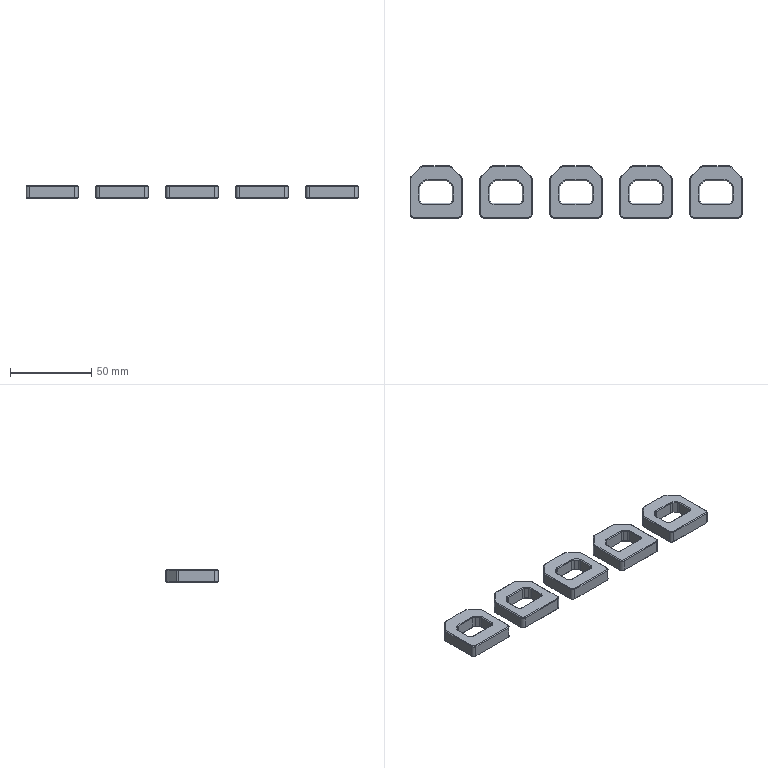NC program | NX | posted with a generic post | part box 204 x 32 x 8 mm
Lines 19 to 988 of 9506:
(ZLEVEL_PROFILE_COPY_1 , TOOL : D10)
N36 T15 M6
N38 G54
N40 G17 G0 G90 X4.9 Y-0.132 S9500 M3
N42 G43 Z30. H15
N44 Z1.5
N46 G94 G1 Y1.888 Z1.394 F1000.
N48 X4.888 Y1.9 Z1.393
N50 X-4.888 Z0.881
N52 X-4.9 Y1.888 Z0.88
N54 Y-1.9 Z0.682
N56 X4.9 Z0.168
N58 Y1.888 Z-0.031
N60 X4.888 Y1.9
N62 X-4.888 Z-0.544
N64 X-4.9 Y1.888 Z-0.545
N66 Y-1.9 Z-0.743
N68 X0. Z-1.
N70 X4.9 F3500.
N72 Y1.888
N74 X4.888 Y1.9
N76 X-4.888
N78 X-4.9 Y1.888
N80 Y-1.9
N82 X0.
N84 X4.9 Z-1.18
N86 Y0.001 Z-1.25
N88 X4.888 Y1.9 Z-1.32
N90 X-4.888 Z-1.68
N92 X-4.9 Y0.635 Z-1.56
N94 Y0. Z-1.5
N96 Y-1.9 Z-1.82
N98 X0. Z-2.
N100 X4.9 Z-2.18
N102 Y0.001 Z-2.25
N104 X4.888 Y1.9 Z-2.32
N106 X-4.888 Z-2.68
N108 X-4.9 Y0.635 Z-2.56
N110 Y0. Z-2.5
N112 Y-1.9 Z-2.82
N114 X0. Z-3.
N116 X4.9 Z-3.18
N118 Y0.001 Z-3.25
N120 X4.888 Y1.9 Z-3.32
N122 X-4.888 Z-3.68
N124 X-4.9 Y0.635 Z-3.56
N126 Y0. Z-3.5
N128 Y-1.9 Z-3.82
N130 X0. Z-4.
N132 X4.9 Z-4.18
N134 Y0.001 Z-4.25
N136 X4.888 Y1.9 Z-4.32
N138 X-4.888 Z-4.68
N140 X-4.9 Y0.635 Z-4.56
N142 Y0. Z-4.5
N144 Y-1.9 Z-4.82
N146 X0. Z-5.
N148 X4.9 Z-5.18
N150 Y0.001 Z-5.25
N152 X4.888 Y1.9 Z-5.32
N154 X-4.888 Z-5.68
N156 X-4.9 Y0.635 Z-5.56
N158 Y0. Z-5.5
N160 Y-1.9 Z-5.82
N162 X0. Z-6.
N164 X4.9 Z-6.18
N166 Y0.001 Z-6.25
N168 X4.888 Y1.9 Z-6.32
N170 X-4.888 Z-6.68
N172 X-4.9 Y0.635 Z-6.56
N174 Y0. Z-6.5
N176 Y-1.9 Z-6.82
N178 X0. Z-7.
N180 X4.9 Z-7.18
N182 Y0.001 Z-7.25
N184 X4.888 Y1.9 Z-7.32
N186 X-4.888 Z-7.68
N188 X-4.9 Y0.635 Z-7.56
N190 Y0. Z-7.5
N192 Y-1.9 Z-7.82
N194 X0. Z-8.
N196 X4.9
N198 Y1.888
N200 X4.888 Y1.9
N202 X-4.888
N204 X-4.9 Y1.888
N206 Y-1.9
N208 X0.
N210 Z-6.5
N212 G0 Z53.
N214 X-38.1 Y-0.132
N216 Z1.5
N218 G1 Y1.888 Z1.394 F1000.
N220 X-38.112 Y1.9 Z1.393
N222 X-47.888 Z0.881
N224 X-47.9 Y1.888 Z0.88
N226 Y-1.9 Z0.682
N228 X-38.1 Z0.168
N230 Y1.888 Z-0.031
N232 X-38.112 Y1.9
N234 X-47.888 Z-0.544
N236 X-47.9 Y1.888 Z-0.545
N238 Y-1.9 Z-0.743
N240 X-43. Z-1.
N242 X-38.1 F3500.
N244 Y1.888
N246 X-38.112 Y1.9
N248 X-47.888
N250 X-47.9 Y1.888
N252 Y-1.9
N254 X-43.
N256 X-38.1 Z-1.18
N258 Y0.002 Z-1.25
N260 X-38.112 Y1.901 Z-1.32
N262 X-47.888 Y1.9 Z-1.68
N264 X-47.9 Y0.635 Z-1.726
N266 Y-1.9 Z-1.82
N268 X-43. Z-2.
N270 X-38.1 Z-2.18
N272 Y0.002 Z-2.25
N274 X-38.112 Y1.901 Z-2.32
N276 X-47.888 Y1.9 Z-2.68
N278 X-47.9 Y0.635 Z-2.726
N280 Y-1.9 Z-2.82
N282 X-43. Z-3.
N284 X-38.1 Z-3.18
N286 Y0.002 Z-3.25
N288 X-38.112 Y1.901 Z-3.32
N290 X-47.888 Y1.9 Z-3.68
N292 X-47.9 Y0.635 Z-3.726
N294 Y-1.9 Z-3.82
N296 X-43. Z-4.
N298 X-38.1 Z-4.18
N300 Y0.002 Z-4.25
N302 X-38.112 Y1.901 Z-4.32
N304 X-47.888 Y1.9 Z-4.68
N306 X-47.9 Y0.635 Z-4.726
N308 Y-1.9 Z-4.82
N310 X-43. Z-5.
N312 X-38.1 Z-5.18
N314 Y0.002 Z-5.25
N316 X-38.112 Y1.901 Z-5.32
N318 X-47.888 Y1.9 Z-5.68
N320 X-47.9 Y0.635 Z-5.726
N322 Y-1.9 Z-5.82
N324 X-43. Z-6.
N326 X-38.1 Z-6.18
N328 Y0.002 Z-6.25
N330 X-38.112 Y1.901 Z-6.32
N332 X-47.888 Y1.9 Z-6.68
N334 X-47.9 Y0.635 Z-6.726
N336 Y-1.9 Z-6.82
N338 X-43. Z-7.
N340 X-38.1 Z-7.18
N342 Y0.002 Z-7.25
N344 X-38.112 Y1.901 Z-7.32
N346 X-47.888 Y1.9 Z-7.68
N348 X-47.9 Y0.635 Z-7.726
N350 Y-1.9 Z-7.82
N352 X-43. Z-8.
N354 X-38.1
N356 Y1.888
N358 X-38.112 Y1.9
N360 X-47.888
N362 X-47.9 Y1.888
N364 Y-1.9
N366 X-43.
N368 Z-6.5
N370 G0 Z53.
N372 X-81.1 Y-0.132
N374 Z1.5
N376 G1 Y1.888 Z1.394 F1000.
N378 X-81.112 Y1.9 Z1.393
N380 X-90.888 Z0.881
N382 X-90.9 Y1.888 Z0.88
N384 Y-1.9 Z0.682
N386 X-81.1 Z0.168
N388 Y1.888 Z-0.031
N390 X-81.112 Y1.9
N392 X-90.888 Z-0.544
N394 X-90.9 Y1.888 Z-0.545
N396 Y-1.9 Z-0.743
N398 X-86. Z-1.
N400 X-81.1 F3500.
N402 Y1.888
N404 X-81.112 Y1.9
N406 X-90.888
N408 X-90.9 Y1.888
N410 Y-1.9
N412 X-86.
N414 X-81.1 Z-1.18
N416 Y0.001 Z-1.25
N418 X-81.112 Y1.9 Z-1.32
N420 X-90.888 Z-1.68
N422 X-90.9 Y0.635 Z-1.56
N424 Y0. Z-1.5
N426 Y-1.9 Z-1.82
N428 X-86. Z-2.
N430 X-81.1 Z-2.18
N432 Y0.001 Z-2.25
N434 X-81.112 Y1.9 Z-2.32
N436 X-90.888 Z-2.68
N438 X-90.9 Y0.635 Z-2.56
N440 Y0. Z-2.5
N442 Y-1.9 Z-2.82
N444 X-86. Z-3.
N446 X-81.1 Z-3.18
N448 Y0.001 Z-3.25
N450 X-81.112 Y1.9 Z-3.32
N452 X-90.888 Z-3.68
N454 X-90.9 Y0.635 Z-3.56
N456 Y0. Z-3.5
N458 Y-1.9 Z-3.82
N460 X-86. Z-4.
N462 X-81.1 Z-4.18
N464 Y0.001 Z-4.25
N466 X-81.112 Y1.9 Z-4.32
N468 X-90.888 Z-4.68
N470 X-90.9 Y0.635 Z-4.56
N472 Y0. Z-4.5
N474 Y-1.9 Z-4.82
N476 X-86. Z-5.
N478 X-81.1 Z-5.18
N480 Y0.001 Z-5.25
N482 X-81.112 Y1.9 Z-5.32
N484 X-90.888 Z-5.68
N486 X-90.9 Y0.635 Z-5.56
N488 Y0. Z-5.5
N490 Y-1.9 Z-5.82
N492 X-86. Z-6.
N494 X-81.1 Z-6.18
N496 Y0.001 Z-6.25
N498 X-81.112 Y1.9 Z-6.32
N500 X-90.888 Z-6.68
N502 X-90.9 Y0.635 Z-6.56
N504 Y0. Z-6.5
N506 Y-1.9 Z-6.82
N508 X-86. Z-7.
N510 X-81.1 Z-7.18
N512 Y0.001 Z-7.25
N514 X-81.112 Y1.9 Z-7.32
N516 X-90.888 Z-7.68
N518 X-90.9 Y0.635 Z-7.56
N520 Y0. Z-7.5
N522 Y-1.9 Z-7.82
N524 X-86. Z-8.
N526 X-81.1
N528 Y1.888
N530 X-81.112 Y1.9
N532 X-90.888
N534 X-90.9 Y1.888
N536 Y-1.9
N538 X-86.
N540 Z-6.5
N542 G0 Z53.
N544 X90.9 Y-0.132
N546 Z1.5
N548 G1 Y1.888 Z1.394 F1000.
N550 X90.888 Y1.9 Z1.393
N552 X81.112 Z0.881
N554 X81.1 Y1.888 Z0.88
N556 Y-1.9 Z0.682
N558 X90.9 Z0.168
N560 Y1.888 Z-0.031
N562 X90.888 Y1.9
N564 X81.112 Z-0.544
N566 X81.1 Y1.888 Z-0.545
N568 Y-1.9 Z-0.743
N570 X86. Z-1.
N572 X90.9 F3500.
N574 Y1.888
N576 X90.888 Y1.9
N578 X81.112
N580 X81.1 Y1.888
N582 Y-1.9
N584 X86.
N586 X90.9 Z-1.18
N588 Y0.002 Z-1.25
N590 X90.888 Y1.901 Z-1.32
N592 X81.112 Y1.9 Z-1.68
N594 X81.1 Y0.635 Z-1.726
N596 Y-1.9 Z-1.82
N598 X86. Z-2.
N600 X90.9 Z-2.18
N602 Y0.002 Z-2.25
N604 X90.888 Y1.901 Z-2.32
N606 X81.112 Y1.9 Z-2.68
N608 X81.1 Y0.635 Z-2.726
N610 Y-1.9 Z-2.82
N612 X86. Z-3.
N614 X90.9 Z-3.18
N616 Y0.002 Z-3.25
N618 X90.888 Y1.901 Z-3.32
N620 X81.112 Y1.9 Z-3.68
N622 X81.1 Y0.635 Z-3.726
N624 Y-1.9 Z-3.82
N626 X86. Z-4.
N628 X90.9 Z-4.18
N630 Y0.002 Z-4.25
N632 X90.888 Y1.901 Z-4.32
N634 X81.112 Y1.9 Z-4.68
N636 X81.1 Y0.635 Z-4.726
N638 Y-1.9 Z-4.82
N640 X86. Z-5.
N642 X90.9 Z-5.18
N644 Y0.002 Z-5.25
N646 X90.888 Y1.901 Z-5.32
N648 X81.112 Y1.9 Z-5.68
N650 X81.1 Y0.635 Z-5.726
N652 Y-1.9 Z-5.82
N654 X86. Z-6.
N656 X90.9 Z-6.18
N658 Y0.002 Z-6.25
N660 X90.888 Y1.901 Z-6.32
N662 X81.112 Y1.9 Z-6.68
N664 X81.1 Y0.635 Z-6.726
N666 Y-1.9 Z-6.82
N668 X86. Z-7.
N670 X90.9 Z-7.18
N672 Y0.002 Z-7.25
N674 X90.888 Y1.901 Z-7.32
N676 X81.112 Y1.9 Z-7.68
N678 X81.1 Y0.635 Z-7.726
N680 Y-1.9 Z-7.82
N682 X86. Z-8.
N684 X90.9
N686 Y1.888
N688 X90.888 Y1.9
N690 X81.112
N692 X81.1 Y1.888
N694 Y-1.9
N696 X86.
N698 Z-6.5
N700 G0 Z53.
N702 X47.9 Y-0.132
N704 Z1.5
N706 G1 Y1.888 Z1.394 F1000.
N708 X47.888 Y1.9 Z1.393
N710 X38.112 Z0.881
N712 X38.1 Y1.888 Z0.88
N714 Y-1.9 Z0.682
N716 X47.9 Z0.168
N718 Y1.888 Z-0.031
N720 X47.888 Y1.9
N722 X38.112 Z-0.544
N724 X38.1 Y1.888 Z-0.545
N726 Y-1.9 Z-0.743
N728 X43. Z-1.
N730 X47.9 F3500.
N732 Y1.888
N734 X47.888 Y1.9
N736 X38.112
N738 X38.1 Y1.888
N740 Y-1.9
N742 X43.
N744 X47.9 Z-1.18
N746 Y0.002 Z-1.25
N748 X47.888 Y1.901 Z-1.32
N750 X38.112 Y1.9 Z-1.68
N752 X38.1 Y0.635 Z-1.726
N754 Y-1.9 Z-1.82
N756 X43. Z-2.
N758 X47.9 Z-2.18
N760 Y0.002 Z-2.25
N762 X47.888 Y1.901 Z-2.32
N764 X38.112 Y1.9 Z-2.68
N766 X38.1 Y0.635 Z-2.726
N768 Y-1.9 Z-2.82
N770 X43. Z-3.
N772 X47.9 Z-3.18
N774 Y0.002 Z-3.25
N776 X47.888 Y1.901 Z-3.32
N778 X38.112 Y1.9 Z-3.68
N780 X38.1 Y0.635 Z-3.726
N782 Y-1.9 Z-3.82
N784 X43. Z-4.
N786 X47.9 Z-4.18
N788 Y0.002 Z-4.25
N790 X47.888 Y1.901 Z-4.32
N792 X38.112 Y1.9 Z-4.68
N794 X38.1 Y0.635 Z-4.726
N796 Y-1.9 Z-4.82
N798 X43. Z-5.
N800 X47.9 Z-5.18
N802 Y0.002 Z-5.25
N804 X47.888 Y1.901 Z-5.32
N806 X38.112 Y1.9 Z-5.68
N808 X38.1 Y0.635 Z-5.726
N810 Y-1.9 Z-5.82
N812 X43. Z-6.
N814 X47.9 Z-6.18
N816 Y0.002 Z-6.25
N818 X47.888 Y1.901 Z-6.32
N820 X38.112 Y1.9 Z-6.68
N822 X38.1 Y0.635 Z-6.726
N824 Y-1.9 Z-6.82
N826 X43. Z-7.
N828 X47.9 Z-7.18
N830 Y0.002 Z-7.25
N832 X47.888 Y1.901 Z-7.32
N834 X38.112 Y1.9 Z-7.68
N836 X38.1 Y0.635 Z-7.726
N838 Y-1.9 Z-7.82
N840 X43. Z-8.
N842 X47.9
N844 Y1.888
N846 X47.888 Y1.9
N848 X38.112
N850 X38.1 Y1.888
N852 Y-1.9
N854 X43.
N856 Z-6.5
N858 G0 Z53.
N860 X64.1 Y8.527
N862 Z1.5
N864 G1 Y-14.653 Z0.285 F1000.
N866 X63.761 Y-16.263 Z0.199
N868 X63.063 Y-17.752 Z0.113
N870 X62.042 Y-19.042 Z0.027
N872 X60.752 Y-20.063 Z-0.06
N874 X59.263 Y-20.761 Z-0.146
N876 X57.653 Y-21.1 Z-0.232
N878 X43. Z-1.
N880 X29. F3500.
N882 G2 X21.9 Y-14. R7.1
N884 G1 Y8.172
N886 G2 X23.98 Y13.192 R7.1
N888 G1 X29.808 Y19.02
N890 G2 X34.828 Y21.1 R7.1
N892 G1 X51.172
N894 G2 X56.192 Y19.02 R7.1
N896 G1 X62.02 Y13.192
N898 G2 X64.1 Y8.172 R7.1
N900 G1 Y-14.
N902 G2 X57. Y-21.1 R7.1
N904 G1 X43.
N906 X29. Z-1.094
N908 X28.381 Y-21.073 Z-1.098
N910 X27.767 Y-20.992 Z-1.102
N912 X27.162 Y-20.858 Z-1.106
N914 X26.572 Y-20.672 Z-1.11
N916 X25.999 Y-20.435 Z-1.114
N918 X25.45 Y-20.149 Z-1.118
N920 X24.928 Y-19.816 Z-1.122
N922 X24.436 Y-19.439 Z-1.127
N924 X23.98 Y-19.02 Z-1.131
N926 X23.561 Y-18.564 Z-1.135
N928 X23.184 Y-18.072 Z-1.139
N930 X22.851 Y-17.55 Z-1.143
N932 X22.565 Y-17.001 Z-1.147
N934 X22.328 Y-16.428 Z-1.151
N936 X22.142 Y-15.838 Z-1.155
N938 X22.008 Y-15.233 Z-1.16
N940 X21.927 Y-14.619 Z-1.164
N942 X21.9 Y-14. Z-1.168
N944 Y8.172 Z-1.316
N946 X21.922 Y8.729 Z-1.32
N948 X21.987 Y9.282 Z-1.323
N950 X22.096 Y9.829 Z-1.327
N952 X22.247 Y10.366 Z-1.331
N954 X22.44 Y10.889 Z-1.335
N956 X22.674 Y11.395 Z-1.338
N958 X22.946 Y11.881 Z-1.342
N960 X23.256 Y12.345 Z-1.346
N962 X23.601 Y12.783 Z-1.349
N964 X23.98 Y13.192 Z-1.353
N966 X29.808 Y19.02 Z-1.408
N968 X30.217 Y19.399 Z-1.412
N970 X30.655 Y19.744 Z-1.416
N972 X31.119 Y20.054 Z-1.419
N974 X31.605 Y20.326 Z-1.423
N976 X32.111 Y20.56 Z-1.427
N978 X32.634 Y20.753 Z-1.431
N980 X33.171 Y20.904 Z-1.434
N982 X33.718 Y21.013 Z-1.438
N984 X34.271 Y21.078 Z-1.442
N986 X34.828 Y21.1 Z-1.445
N988 X51.172 Z-1.555
N990 X51.729 Y21.078 Z-1.558
N992 X52.282 Y21.013 Z-1.562
N994 X52.829 Y20.904 Z-1.566
N996 X53.366 Y20.753 Z-1.569
N998 X53.889 Y20.56 Z-1.573
N1000 X54.395 Y20.326 Z-1.577
N1002 X54.881 Y20.054 Z-1.581
N1004 X55.345 Y19.744 Z-1.584
N1006 X55.783 Y19.399 Z-1.588
N1008 X56.192 Y19.02 Z-1.592
N1010 X62.02 Y13.192 Z-1.647
N1012 X62.399 Y12.783 Z-1.651
N1014 X62.744 Y12.345 Z-1.654
N1016 X63.054 Y11.881 Z-1.658
N1018 X63.326 Y11.395 Z-1.662
N1020 X63.56 Y10.889 Z-1.665
N1022 X63.753 Y10.366 Z-1.669
N1024 X63.904 Y9.829 Z-1.673
N1026 X64.013 Y9.282 Z-1.677
N1028 X64.078 Y8.729 Z-1.68
N1030 X64.1 Y8.172 Z-1.684
N1032 Y-14. Z-1.832
N1034 X64.073 Y-14.619 Z-1.836
N1036 X63.992 Y-15.233 Z-1.84
N1038 X63.858 Y-15.838 Z-1.845
N1040 X63.672 Y-16.428 Z-1.849
N1042 X63.435 Y-17.001 Z-1.853
N1044 X63.149 Y-17.55 Z-1.857
N1046 X62.816 Y-18.072 Z-1.861
N1048 X62.439 Y-18.564 Z-1.865
N1050 X62.02 Y-19.02 Z-1.869
N1052 X61.564 Y-19.439 Z-1.873
N1054 X61.072 Y-19.816 Z-1.878
N1056 X60.55 Y-20.149 Z-1.882
N1058 X60.001 Y-20.435 Z-1.886
N1060 X59.428 Y-20.672 Z-1.89
N1062 X58.838 Y-20.858 Z-1.894
N1064 X58.233 Y-20.992 Z-1.898
N1066 X57.619 Y-21.073 Z-1.902
N1068 X57. Y-21.1 Z-1.906
N1070 X43. Z-2.
N1072 X29. Z-2.094
N1074 X28.381 Y-21.073 Z-2.098
N1076 X27.767 Y-20.992 Z-2.102
N1078 X27.162 Y-20.858 Z-2.106
N1080 X26.572 Y-20.672 Z-2.11
N1082 X25.999 Y-20.435 Z-2.114
N1084 X25.45 Y-20.149 Z-2.118
N1086 X24.928 Y-19.816 Z-2.122
N1088 X24.436 Y-19.439 Z-2.127
N1090 X23.98 Y-19.02 Z-2.131
N1092 X23.561 Y-18.564 Z-2.135
N1094 X23.184 Y-18.072 Z-2.139
N1096 X22.851 Y-17.55 Z-2.143
N1098 X22.565 Y-17.001 Z-2.147
N1100 X22.328 Y-16.428 Z-2.151
N1102 X22.142 Y-15.838 Z-2.155
N1104 X22.008 Y-15.233 Z-2.16
N1106 X21.927 Y-14.619 Z-2.164
N1108 X21.9 Y-14. Z-2.168
N1110 Y8.172 Z-2.316
N1112 X21.922 Y8.729 Z-2.32
N1114 X21.987 Y9.282 Z-2.323
N1116 X22.096 Y9.829 Z-2.327
N1118 X22.247 Y10.366 Z-2.331
N1120 X22.44 Y10.889 Z-2.335
N1122 X22.674 Y11.395 Z-2.338
N1124 X22.946 Y11.881 Z-2.342
N1126 X23.256 Y12.345 Z-2.346
N1128 X23.601 Y12.783 Z-2.349
N1130 X23.98 Y13.192 Z-2.353
N1132 X29.808 Y19.02 Z-2.408
N1134 X30.217 Y19.399 Z-2.412
N1136 X30.655 Y19.744 Z-2.416
N1138 X31.119 Y20.054 Z-2.419
N1140 X31.605 Y20.326 Z-2.423
N1142 X32.111 Y20.56 Z-2.427
N1144 X32.634 Y20.753 Z-2.431
N1146 X33.171 Y20.904 Z-2.434
N1148 X33.718 Y21.013 Z-2.438
N1150 X34.271 Y21.078 Z-2.442
N1152 X34.828 Y21.1 Z-2.445
N1154 X51.172 Z-2.555
N1156 X51.729 Y21.078 Z-2.558
N1158 X52.282 Y21.013 Z-2.562
N1160 X52.829 Y20.904 Z-2.566
N1162 X53.366 Y20.753 Z-2.569
N1164 X53.889 Y20.56 Z-2.573
N1166 X54.395 Y20.326 Z-2.577
N1168 X54.881 Y20.054 Z-2.581
N1170 X55.345 Y19.744 Z-2.584
N1172 X55.783 Y19.399 Z-2.588
N1174 X56.192 Y19.02 Z-2.592
N1176 X62.02 Y13.192 Z-2.647
N1178 X62.399 Y12.783 Z-2.651
N1180 X62.744 Y12.345 Z-2.654
N1182 X63.054 Y11.881 Z-2.658
N1184 X63.326 Y11.395 Z-2.662
N1186 X63.56 Y10.889 Z-2.665
N1188 X63.753 Y10.366 Z-2.669
N1190 X63.904 Y9.829 Z-2.673
N1192 X64.013 Y9.282 Z-2.677
N1194 X64.078 Y8.729 Z-2.68
N1196 X64.1 Y8.172 Z-2.684
N1198 Y-14. Z-2.832
N1200 X64.073 Y-14.619 Z-2.836
N1202 X63.992 Y-15.233 Z-2.84
N1204 X63.858 Y-15.838 Z-2.845
N1206 X63.672 Y-16.428 Z-2.849
N1208 X63.435 Y-17.001 Z-2.853
N1210 X63.149 Y-17.55 Z-2.857
N1212 X62.816 Y-18.072 Z-2.861
N1214 X62.439 Y-18.564 Z-2.865
N1216 X62.02 Y-19.02 Z-2.869
N1218 X61.564 Y-19.439 Z-2.873
N1220 X61.072 Y-19.816 Z-2.878
N1222 X60.55 Y-20.149 Z-2.882
N1224 X60.001 Y-20.435 Z-2.886
N1226 X59.428 Y-20.672 Z-2.89
N1228 X58.838 Y-20.858 Z-2.894
N1230 X58.233 Y-20.992 Z-2.898
N1232 X57.619 Y-21.073 Z-2.902
N1234 X57. Y-21.1 Z-2.906
N1236 X43. Z-3.
N1238 X29. Z-3.094
N1240 X28.381 Y-21.073 Z-3.098
N1242 X27.767 Y-20.992 Z-3.102
N1244 X27.162 Y-20.858 Z-3.106
N1246 X26.572 Y-20.672 Z-3.11
N1248 X25.999 Y-20.435 Z-3.114
N1250 X25.45 Y-20.149 Z-3.118
N1252 X24.928 Y-19.816 Z-3.122
N1254 X24.436 Y-19.439 Z-3.127
N1256 X23.98 Y-19.02 Z-3.131
N1258 X23.561 Y-18.564 Z-3.135
N1260 X23.184 Y-18.072 Z-3.139
N1262 X22.851 Y-17.55 Z-3.143
N1264 X22.565 Y-17.001 Z-3.147
N1266 X22.328 Y-16.428 Z-3.151
N1268 X22.142 Y-15.838 Z-3.155
N1270 X22.008 Y-15.233 Z-3.16
N1272 X21.927 Y-14.619 Z-3.164
N1274 X21.9 Y-14. Z-3.168
N1276 Y8.172 Z-3.316
N1278 X21.922 Y8.729 Z-3.32
N1280 X21.987 Y9.282 Z-3.323
N1282 X22.096 Y9.829 Z-3.327
N1284 X22.247 Y10.366 Z-3.331
N1286 X22.44 Y10.889 Z-3.335
N1288 X22.674 Y11.395 Z-3.338
N1290 X22.946 Y11.881 Z-3.342
N1292 X23.256 Y12.345 Z-3.346
N1294 X23.601 Y12.783 Z-3.349
N1296 X23.98 Y13.192 Z-3.353
N1298 X29.808 Y19.02 Z-3.408
N1300 X30.217 Y19.399 Z-3.412
N1302 X30.655 Y19.744 Z-3.416
N1304 X31.119 Y20.054 Z-3.419
N1306 X31.605 Y20.326 Z-3.423
N1308 X32.111 Y20.56 Z-3.427
N1310 X32.634 Y20.753 Z-3.431
N1312 X33.171 Y20.904 Z-3.434
N1314 X33.718 Y21.013 Z-3.438
N1316 X34.271 Y21.078 Z-3.442
N1318 X34.828 Y21.1 Z-3.445
N1320 X51.172 Z-3.555
N1322 X51.729 Y21.078 Z-3.558
N1324 X52.282 Y21.013 Z-3.562
N1326 X52.829 Y20.904 Z-3.566
N1328 X53.366 Y20.753 Z-3.569
N1330 X53.889 Y20.56 Z-3.573
N1332 X54.395 Y20.326 Z-3.577
N1334 X54.881 Y20.054 Z-3.581
N1336 X55.345 Y19.744 Z-3.584
N1338 X55.783 Y19.399 Z-3.588
N1340 X56.192 Y19.02 Z-3.592
N1342 X62.02 Y13.192 Z-3.647
N1344 X62.399 Y12.783 Z-3.651
N1346 X62.744 Y12.345 Z-3.654
N1348 X63.054 Y11.881 Z-3.658
N1350 X63.326 Y11.395 Z-3.662
N1352 X63.56 Y10.889 Z-3.665
N1354 X63.753 Y10.366 Z-3.669
N1356 X63.904 Y9.829 Z-3.673
N1358 X64.013 Y9.282 Z-3.677
N1360 X64.078 Y8.729 Z-3.68
N1362 X64.1 Y8.172 Z-3.684
N1364 Y-14. Z-3.832
N1366 X64.073 Y-14.619 Z-3.836
N1368 X63.992 Y-15.233 Z-3.84
N1370 X63.858 Y-15.838 Z-3.845
N1372 X63.672 Y-16.428 Z-3.849
N1374 X63.435 Y-17.001 Z-3.853
N1376 X63.149 Y-17.55 Z-3.857
N1378 X62.816 Y-18.072 Z-3.861
N1380 X62.439 Y-18.564 Z-3.865
N1382 X62.02 Y-19.02 Z-3.869
N1384 X61.564 Y-19.439 Z-3.873
N1386 X61.072 Y-19.816 Z-3.878
N1388 X60.55 Y-20.149 Z-3.882
N1390 X60.001 Y-20.435 Z-3.886
N1392 X59.428 Y-20.672 Z-3.89
N1394 X58.838 Y-20.858 Z-3.894
N1396 X58.233 Y-20.992 Z-3.898
N1398 X57.619 Y-21.073 Z-3.902
N1400 X57. Y-21.1 Z-3.906
N1402 X43. Z-4.
N1404 X29. Z-4.094
N1406 X28.381 Y-21.073 Z-4.098
N1408 X27.767 Y-20.992 Z-4.102
N1410 X27.162 Y-20.858 Z-4.106
N1412 X26.572 Y-20.672 Z-4.11
N1414 X25.999 Y-20.435 Z-4.114
N1416 X25.45 Y-20.149 Z-4.118
N1418 X24.928 Y-19.816 Z-4.122
N1420 X24.436 Y-19.439 Z-4.127
N1422 X23.98 Y-19.02 Z-4.131
N1424 X23.561 Y-18.564 Z-4.135
N1426 X23.184 Y-18.072 Z-4.139
N1428 X22.851 Y-17.55 Z-4.143
N1430 X22.565 Y-17.001 Z-4.147
N1432 X22.328 Y-16.428 Z-4.151
N1434 X22.142 Y-15.838 Z-4.155
N1436 X22.008 Y-15.233 Z-4.16
N1438 X21.927 Y-14.619 Z-4.164
N1440 X21.9 Y-14. Z-4.168
N1442 Y8.172 Z-4.316
N1444 X21.922 Y8.729 Z-4.32
N1446 X21.987 Y9.282 Z-4.323
N1448 X22.096 Y9.829 Z-4.327
N1450 X22.247 Y10.366 Z-4.331
N1452 X22.44 Y10.889 Z-4.335
N1454 X22.674 Y11.395 Z-4.338
N1456 X22.946 Y11.881 Z-4.342
N1458 X23.256 Y12.345 Z-4.346
N1460 X23.601 Y12.783 Z-4.349
N1462 X23.98 Y13.192 Z-4.353
N1464 X29.808 Y19.02 Z-4.408
N1466 X30.217 Y19.399 Z-4.412
N1468 X30.655 Y19.744 Z-4.416
N1470 X31.119 Y20.054 Z-4.419
N1472 X31.605 Y20.326 Z-4.423
N1474 X32.111 Y20.56 Z-4.427
N1476 X32.634 Y20.753 Z-4.431
N1478 X33.171 Y20.904 Z-4.434
N1480 X33.718 Y21.013 Z-4.438
N1482 X34.271 Y21.078 Z-4.442
N1484 X34.828 Y21.1 Z-4.445
N1486 X51.172 Z-4.555
N1488 X51.729 Y21.078 Z-4.558
N1490 X52.282 Y21.013 Z-4.562
N1492 X52.829 Y20.904 Z-4.566
N1494 X53.366 Y20.753 Z-4.569
N1496 X53.889 Y20.56 Z-4.573
N1498 X54.395 Y20.326 Z-4.577
N1500 X54.881 Y20.054 Z-4.581
N1502 X55.345 Y19.744 Z-4.584
N1504 X55.783 Y19.399 Z-4.588
N1506 X56.192 Y19.02 Z-4.592
N1508 X62.02 Y13.192 Z-4.647
N1510 X62.399 Y12.783 Z-4.651
N1512 X62.744 Y12.345 Z-4.654
N1514 X63.054 Y11.881 Z-4.658
N1516 X63.326 Y11.395 Z-4.662
N1518 X63.56 Y10.889 Z-4.665
N1520 X63.753 Y10.366 Z-4.669
N1522 X63.904 Y9.829 Z-4.673
N1524 X64.013 Y9.282 Z-4.677
N1526 X64.078 Y8.729 Z-4.68
N1528 X64.1 Y8.172 Z-4.684
N1530 Y-14. Z-4.832
N1532 X64.073 Y-14.619 Z-4.836
N1534 X63.992 Y-15.233 Z-4.84
N1536 X63.858 Y-15.838 Z-4.845
N1538 X63.672 Y-16.428 Z-4.849
N1540 X63.435 Y-17.001 Z-4.853
N1542 X63.149 Y-17.55 Z-4.857
N1544 X62.816 Y-18.072 Z-4.861
N1546 X62.439 Y-18.564 Z-4.865
N1548 X62.02 Y-19.02 Z-4.869
N1550 X61.564 Y-19.439 Z-4.873
N1552 X61.072 Y-19.816 Z-4.878
N1554 X60.55 Y-20.149 Z-4.882
N1556 X60.001 Y-20.435 Z-4.886
N1558 X59.428 Y-20.672 Z-4.89
N1560 X58.838 Y-20.858 Z-4.894
N1562 X58.233 Y-20.992 Z-4.898
N1564 X57.619 Y-21.073 Z-4.902
N1566 X57. Y-21.1 Z-4.906
N1568 X43. Z-5.
N1570 X29. Z-5.094
N1572 X28.381 Y-21.073 Z-5.098
N1574 X27.767 Y-20.992 Z-5.102
N1576 X27.162 Y-20.858 Z-5.106
N1578 X26.572 Y-20.672 Z-5.11
N1580 X25.999 Y-20.435 Z-5.114
N1582 X25.45 Y-20.149 Z-5.118
N1584 X24.928 Y-19.816 Z-5.122
N1586 X24.436 Y-19.439 Z-5.127
N1588 X23.98 Y-19.02 Z-5.131
N1590 X23.561 Y-18.564 Z-5.135
N1592 X23.184 Y-18.072 Z-5.139
N1594 X22.851 Y-17.55 Z-5.143
N1596 X22.565 Y-17.001 Z-5.147
N1598 X22.328 Y-16.428 Z-5.151
N1600 X22.142 Y-15.838 Z-5.155
N1602 X22.008 Y-15.233 Z-5.16
N1604 X21.927 Y-14.619 Z-5.164
N1606 X21.9 Y-14. Z-5.168
N1608 Y8.172 Z-5.316
N1610 X21.922 Y8.729 Z-5.32
N1612 X21.987 Y9.282 Z-5.323
N1614 X22.096 Y9.829 Z-5.327
N1616 X22.247 Y10.366 Z-5.331
N1618 X22.44 Y10.889 Z-5.335
N1620 X22.674 Y11.395 Z-5.338
N1622 X22.946 Y11.881 Z-5.342
N1624 X23.256 Y12.345 Z-5.346
N1626 X23.601 Y12.783 Z-5.349
N1628 X23.98 Y13.192 Z-5.353
N1630 X29.808 Y19.02 Z-5.408
N1632 X30.217 Y19.399 Z-5.412
N1634 X30.655 Y19.744 Z-5.416
N1636 X31.119 Y20.054 Z-5.419
N1638 X31.605 Y20.326 Z-5.423
N1640 X32.111 Y20.56 Z-5.427
N1642 X32.634 Y20.753 Z-5.431
N1644 X33.171 Y20.904 Z-5.434
N1646 X33.718 Y21.013 Z-5.438
N1648 X34.271 Y21.078 Z-5.442
N1650 X34.828 Y21.1 Z-5.445
N1652 X51.172 Z-5.555
N1654 X51.729 Y21.078 Z-5.558
N1656 X52.282 Y21.013 Z-5.562
N1658 X52.829 Y20.904 Z-5.566
N1660 X53.366 Y20.753 Z-5.569
N1662 X53.889 Y20.56 Z-5.573
N1664 X54.395 Y20.326 Z-5.577
N1666 X54.881 Y20.054 Z-5.581
N1668 X55.345 Y19.744 Z-5.584
N1670 X55.783 Y19.399 Z-5.588
N1672 X56.192 Y19.02 Z-5.592
N1674 X62.02 Y13.192 Z-5.647
N1676 X62.399 Y12.783 Z-5.651
N1678 X62.744 Y12.345 Z-5.654
N1680 X63.054 Y11.881 Z-5.658
N1682 X63.326 Y11.395 Z-5.662
N1684 X63.56 Y10.889 Z-5.665
N1686 X63.753 Y10.366 Z-5.669
N1688 X63.904 Y9.829 Z-5.673
N1690 X64.013 Y9.282 Z-5.677
N1692 X64.078 Y8.729 Z-5.68
N1694 X64.1 Y8.172 Z-5.684
N1696 Y-14. Z-5.832
N1698 X64.073 Y-14.619 Z-5.836
N1700 X63.992 Y-15.233 Z-5.84
N1702 X63.858 Y-15.838 Z-5.845
N1704 X63.672 Y-16.428 Z-5.849
N1706 X63.435 Y-17.001 Z-5.853
N1708 X63.149 Y-17.55 Z-5.857
N1710 X62.816 Y-18.072 Z-5.861
N1712 X62.439 Y-18.564 Z-5.865
N1714 X62.02 Y-19.02 Z-5.869
N1716 X61.564 Y-19.439 Z-5.873
N1718 X61.072 Y-19.816 Z-5.878
N1720 X60.55 Y-20.149 Z-5.882
N1722 X60.001 Y-20.435 Z-5.886
N1724 X59.428 Y-20.672 Z-5.89
N1726 X58.838 Y-20.858 Z-5.894
N1728 X58.233 Y-20.992 Z-5.898
N1730 X57.619 Y-21.073 Z-5.902
N1732 X57. Y-21.1 Z-5.906
N1734 X43. Z-6.
N1736 X29. Z-6.094
N1738 X28.381 Y-21.073 Z-6.098
N1740 X27.767 Y-20.992 Z-6.102
N1742 X27.162 Y-20.858 Z-6.106
N1744 X26.572 Y-20.672 Z-6.11
N1746 X25.999 Y-20.435 Z-6.114
N1748 X25.45 Y-20.149 Z-6.118
N1750 X24.928 Y-19.816 Z-6.122
N1752 X24.436 Y-19.439 Z-6.127
N1754 X23.98 Y-19.02 Z-6.131
N1756 X23.561 Y-18.564 Z-6.135
N1758 X23.184 Y-18.072 Z-6.139
N1760 X22.851 Y-17.55 Z-6.143
N1762 X22.565 Y-17.001 Z-6.147
N1764 X22.328 Y-16.428 Z-6.151
N1766 X22.142 Y-15.838 Z-6.155
N1768 X22.008 Y-15.233 Z-6.16
N1770 X21.927 Y-14.619 Z-6.164
N1772 X21.9 Y-14. Z-6.168
N1774 Y8.172 Z-6.316
N1776 X21.922 Y8.729 Z-6.32
N1778 X21.987 Y9.282 Z-6.323
N1780 X22.096 Y9.829 Z-6.327
N1782 X22.247 Y10.366 Z-6.331
N1784 X22.44 Y10.889 Z-6.335
N1786 X22.674 Y11.395 Z-6.338
N1788 X22.946 Y11.881 Z-6.342
N1790 X23.256 Y12.345 Z-6.346
N1792 X23.601 Y12.783 Z-6.349
N1794 X23.98 Y13.192 Z-6.353
N1796 X29.808 Y19.02 Z-6.408
N1798 X30.217 Y19.399 Z-6.412
N1800 X30.655 Y19.744 Z-6.416
N1802 X31.119 Y20.054 Z-6.419
N1804 X31.605 Y20.326 Z-6.423
N1806 X32.111 Y20.56 Z-6.427
N1808 X32.634 Y20.753 Z-6.431
N1810 X33.171 Y20.904 Z-6.434
N1812 X33.718 Y21.013 Z-6.438
N1814 X34.271 Y21.078 Z-6.442
N1816 X34.828 Y21.1 Z-6.445
N1818 X51.172 Z-6.555
N1820 X51.729 Y21.078 Z-6.558
N1822 X52.282 Y21.013 Z-6.562
N1824 X52.829 Y20.904 Z-6.566
N1826 X53.366 Y20.753 Z-6.569
N1828 X53.889 Y20.56 Z-6.573
N1830 X54.395 Y20.326 Z-6.577
N1832 X54.881 Y20.054 Z-6.581
N1834 X55.345 Y19.744 Z-6.584
N1836 X55.783 Y19.399 Z-6.588
N1838 X56.192 Y19.02 Z-6.592
N1840 X62.02 Y13.192 Z-6.647
N1842 X62.399 Y12.783 Z-6.651
N1844 X62.744 Y12.345 Z-6.654
N1846 X63.054 Y11.881 Z-6.658
N1848 X63.326 Y11.395 Z-6.662
N1850 X63.56 Y10.889 Z-6.665
N1852 X63.753 Y10.366 Z-6.669
N1854 X63.904 Y9.829 Z-6.673
N1856 X64.013 Y9.282 Z-6.677
N1858 X64.078 Y8.729 Z-6.68
N1860 X64.1 Y8.172 Z-6.684
N1862 Y-14. Z-6.832
N1864 X64.073 Y-14.619 Z-6.836
N1866 X63.992 Y-15.233 Z-6.84
N1868 X63.858 Y-15.838 Z-6.845
N1870 X63.672 Y-16.428 Z-6.849
N1872 X63.435 Y-17.001 Z-6.853
N1874 X63.149 Y-17.55 Z-6.857
N1876 X62.816 Y-18.072 Z-6.861
N1878 X62.439 Y-18.564 Z-6.865
N1880 X62.02 Y-19.02 Z-6.869
N1882 X61.564 Y-19.439 Z-6.873
N1884 X61.072 Y-19.816 Z-6.878
N1886 X60.55 Y-20.149 Z-6.882
N1888 X60.001 Y-20.435 Z-6.886
N1890 X59.428 Y-20.672 Z-6.89
N1892 X58.838 Y-20.858 Z-6.894
N1894 X58.233 Y-20.992 Z-6.898
N1896 X57.619 Y-21.073 Z-6.902
N1898 X57. Y-21.1 Z-6.906
N1900 X43. Z-7.
N1902 X29. Z-7.094
N1904 X28.381 Y-21.073 Z-7.098
N1906 X27.767 Y-20.992 Z-7.102
N1908 X27.162 Y-20.858 Z-7.106
N1910 X26.572 Y-20.672 Z-7.11
N1912 X25.999 Y-20.435 Z-7.114
N1914 X25.45 Y-20.149 Z-7.118
N1916 X24.928 Y-19.816 Z-7.122
N1918 X24.436 Y-19.439 Z-7.127
N1920 X23.98 Y-19.02 Z-7.131
N1922 X23.561 Y-18.564 Z-7.135
N1924 X23.184 Y-18.072 Z-7.139
N1926 X22.851 Y-17.55 Z-7.143
N1928 X22.565 Y-17.001 Z-7.147
N1930 X22.328 Y-16.428 Z-7.151
N1932 X22.142 Y-15.838 Z-7.155
N1934 X22.008 Y-15.233 Z-7.16
N1936 X21.927 Y-14.619 Z-7.164
N1938 X21.9 Y-14. Z-7.168
N1940 Y8.172 Z-7.316
N1942 X21.922 Y8.729 Z-7.32
N1944 X21.987 Y9.282 Z-7.323
N1946 X22.096 Y9.829 Z-7.327
N1948 X22.247 Y10.366 Z-7.331
N1950 X22.44 Y10.889 Z-7.335
N1952 X22.674 Y11.395 Z-7.338
N1954 X22.946 Y11.881 Z-7.342
N1956 X23.256 Y12.345 Z-7.346
N1958 X23.601 Y12.783 Z-7.349
N1960 X23.98 Y13.192 Z-7.353
N1962 X29.808 Y19.02 Z-7.408
N1964 X30.217 Y19.399 Z-7.412
N1966 X30.655 Y19.744 Z-7.416
N1968 X31.119 Y20.054 Z-7.419